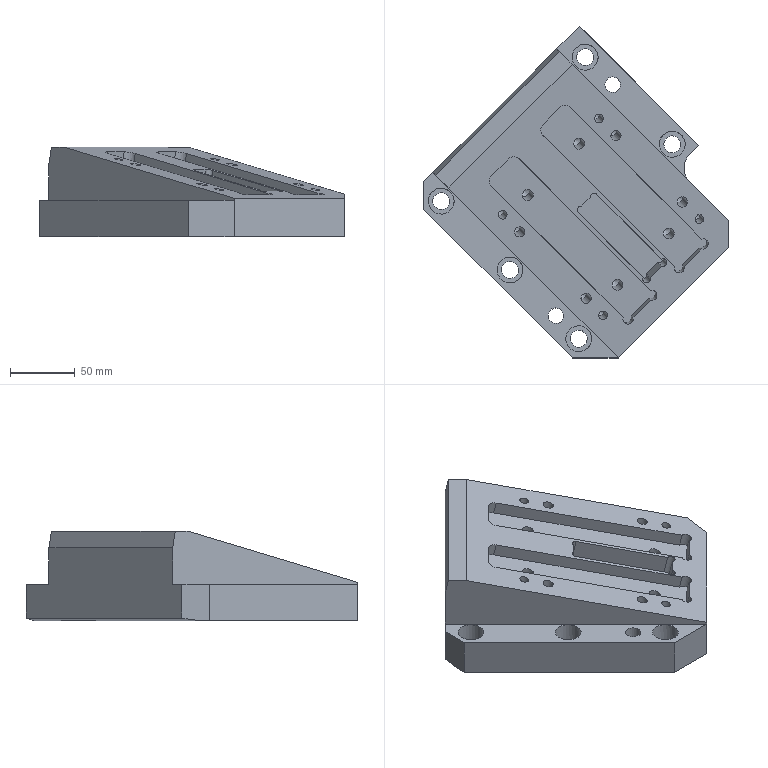Part | STEP file | gslz 2016.10.28-13_id1542_x_t | 1 solid | 86 faces | box 234.759 x 255.973 x 69 mm | volume 1431737 mm3 | plane 37 | cylinder 37 | cone 12 | commonest cylinder face diameters 8 x8 12 x6 13 x5 20 x5 6 x4 6.8 x4